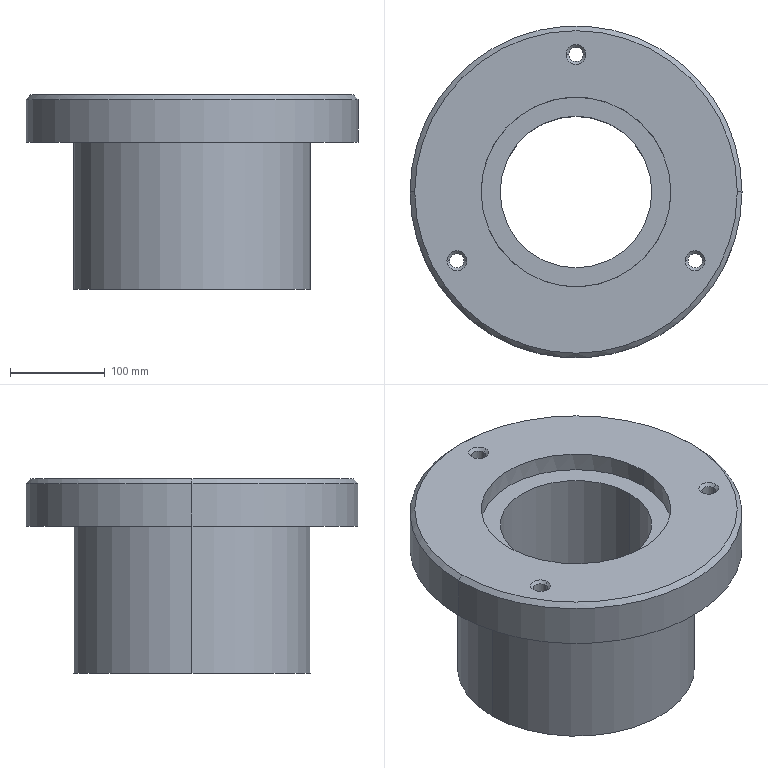Part | SolidWorks | features BaseBody 1 | 1 solid | 26 faces | box 350 x 350 x 205 mm | volume 8030304 mm3 | cylinder 14 | cone 8 | plane 4 | commonest cylinder face diameters 15 x6 160 x2 200 x2 250 x2 350 x2
STEP:
#1=CARTESIAN_POINT('',(165.077,953.249,590.107));
#2=VERTEX_POINT('',#1);
#3=CARTESIAN_POINT('',(165.077,953.249,610.107));
#4=VERTEX_POINT('',#3);
#5=CARTESIAN_POINT('',(165.077,953.249,590.107));
#6=DIRECTION('',(0.,0.,1.));
#7=VECTOR('',#6,1000.);
#8=LINE('',#5,#7);
#9=EDGE_CURVE('',#2,#4,#8,.T.);
#10=ORIENTED_EDGE('',*,*,#9,.F.);
#11=CARTESIAN_POINT('',(365.077,953.249,590.107));
#12=VERTEX_POINT('',#11);
#13=CARTESIAN_POINT('',(265.077,953.249,590.107));
#14=DIRECTION('',(0.,0.,-1.));
#15=DIRECTION('',(-0.9237,-0.383,0.));
#16=AXIS2_PLACEMENT_3D('',#13,#14,#15);
#17=CIRCLE('',#16,100.);
#18=EDGE_CURVE('',#2,#12,#17,.T.);
#19=ORIENTED_EDGE('',*,*,#18,.T.);
#20=CARTESIAN_POINT('',(365.077,953.249,610.107));
#21=VERTEX_POINT('',#20);
#22=CARTESIAN_POINT('',(365.077,953.249,590.107));
#23=DIRECTION('',(0.,0.,1.));
#24=VECTOR('',#23,1000.);
#25=LINE('',#22,#24);
#26=EDGE_CURVE('',#12,#21,#25,.T.);
#27=ORIENTED_EDGE('',*,*,#26,.T.);
#28=CARTESIAN_POINT('',(365.077,953.249,610.107));
#29=CARTESIAN_POINT('',(365.077,959.794,610.107));
#30=CARTESIAN_POINT('',(364.432,966.339,610.107));
#31=CARTESIAN_POINT('',(361.879,979.177,610.107));
#32=CARTESIAN_POINT('',(359.97,985.471,610.107));
#33=CARTESIAN_POINT('',(354.96,997.564,610.107));
#34=CARTESIAN_POINT('',(351.86,1003.364,610.107));
#35=CARTESIAN_POINT('',(344.588,1014.248,610.107));
#36=CARTESIAN_POINT('',(340.416,1019.332,610.107));
#37=CARTESIAN_POINT('',(331.16,1028.588,610.107));
#38=CARTESIAN_POINT('',(326.076,1032.76,610.107));
#39=CARTESIAN_POINT('',(315.192,1040.032,610.107));
#40=CARTESIAN_POINT('',(309.392,1043.132,610.107));
#41=CARTESIAN_POINT('',(297.298,1048.142,610.107));
#42=CARTESIAN_POINT('',(291.005,1050.051,610.107));
#43=CARTESIAN_POINT('',(278.167,1052.604,610.107));
#44=CARTESIAN_POINT('',(271.622,1053.249,610.107));
#45=CARTESIAN_POINT('',(258.532,1053.249,610.107));
#46=CARTESIAN_POINT('',(251.987,1052.604,610.107));
#47=CARTESIAN_POINT('',(239.149,1050.051,610.107));
#48=CARTESIAN_POINT('',(232.855,1048.142,610.107));
#49=CARTESIAN_POINT('',(220.762,1043.132,610.107));
#50=CARTESIAN_POINT('',(214.962,1040.032,610.107));
#51=CARTESIAN_POINT('',(204.078,1032.76,610.107));
#52=CARTESIAN_POINT('',(198.994,1028.588,610.107));
#53=CARTESIAN_POINT('',(189.738,1019.332,610.107));
#54=CARTESIAN_POINT('',(185.566,1014.248,610.107));
#55=CARTESIAN_POINT('',(178.294,1003.364,610.107));
#56=CARTESIAN_POINT('',(175.194,997.564,610.107));
#57=CARTESIAN_POINT('',(170.184,985.471,610.107));
#58=CARTESIAN_POINT('',(168.275,979.177,610.107));
#59=CARTESIAN_POINT('',(165.722,966.339,610.107));
#60=CARTESIAN_POINT('',(165.077,959.794,610.107));
#61=CARTESIAN_POINT('',(165.077,953.249,610.107));
#62=B_SPLINE_CURVE_WITH_KNOTS('',3,(#28,#29,#30,#31,#32,#33,#34,#35,#36,#37,#38,#39,#40,#41,#42,#43,#44,#45,#46,#47,#48,#49,#50,#51,#52,#53,#54,#55,#56,#57,#58,#59,#60,#61),.UNSPECIFIED.,.F.,.F.,(4,2,2,2,2,2,2,2,2,2,2,2,2,2,2,2,4),(0.,0.0625,0.125,0.1875,0.25,0.3125,0.375,0.4375,0.5,0.5625,0.625,0.6875,0.75,0.8125,0.875,0.9375,1.),.UNSPECIFIED.);
#63=EDGE_CURVE('',#21,#4,#62,.T.);
#64=ORIENTED_EDGE('',*,*,#63,.T.);
#65=EDGE_LOOP('',(#10,#19,#27,#64));
#66=FACE_OUTER_BOUND('',#65,.T.);
#67=CARTESIAN_POINT('',(265.077,953.249,590.107));
#68=DIRECTION('',(0.,0.,1.));
#69=DIRECTION('',(1.,0.,0.));
#70=AXIS2_PLACEMENT_3D('',#67,#68,#69);
#71=CYLINDRICAL_SURFACE('',#70,100.);
#72=ADVANCED_FACE('',(#66),#71,.F.);
#73=CARTESIAN_POINT('',(345.077,953.249,590.107));
#74=VERTEX_POINT('',#73);
#75=CARTESIAN_POINT('',(185.077,953.249,590.107));
#76=VERTEX_POINT('',#75);
#77=CARTESIAN_POINT('',(265.077,953.249,590.107));
#78=DIRECTION('',(0.,0.,1.));
#79=DIRECTION('',(-1.,0.,0.));
#80=AXIS2_PLACEMENT_3D('',#77,#78,#79);
#81=CIRCLE('',#80,80.);
#82=EDGE_CURVE('',#74,#76,#81,.T.);
#83=ORIENTED_EDGE('',*,*,#82,.F.);
#84=CARTESIAN_POINT('',(265.077,953.249,590.107));
#85=DIRECTION('',(0.,0.,1.));
#86=DIRECTION('',(-1.,0.,0.));
#87=AXIS2_PLACEMENT_3D('',#84,#85,#86);
#88=CIRCLE('',#87,80.);
#89=EDGE_CURVE('',#76,#74,#88,.T.);
#90=ORIENTED_EDGE('',*,*,#89,.F.);
#91=EDGE_LOOP('',(#83,#90));
#92=FACE_BOUND('',#91,.T.);
#93=CARTESIAN_POINT('',(265.077,953.249,590.107));
#94=DIRECTION('',(0.,0.,-1.));
#95=DIRECTION('',(-0.9237,-0.383,0.));
#96=AXIS2_PLACEMENT_3D('',#93,#94,#95);
#97=CIRCLE('',#96,100.);
#98=EDGE_CURVE('',#12,#2,#97,.T.);
#99=ORIENTED_EDGE('',*,*,#98,.F.);
#100=ORIENTED_EDGE('',*,*,#18,.F.);
#101=EDGE_LOOP('',(#99,#100));
#102=FACE_OUTER_BOUND('',#101,.T.);
#103=CARTESIAN_POINT('',(265.077,953.249,590.107));
#104=DIRECTION('',(0.,0.,-1.));
#105=DIRECTION('',(0.,-1.,0.));
#106=AXIS2_PLACEMENT_3D('',#103,#104,#105);
#107=PLANE('',#106);
#108=ADVANCED_FACE('',(#92,#102),#107,.F.);
#109=CARTESIAN_POINT('',(345.077,953.249,405.107));
#110=VERTEX_POINT('',#109);
#111=CARTESIAN_POINT('',(345.077,953.249,560.107));
#112=DIRECTION('',(0.,0.,-1.));
#113=VECTOR('',#112,1000.);
#114=LINE('',#111,#113);
#115=EDGE_CURVE('',#74,#110,#114,.T.);
#116=ORIENTED_EDGE('',*,*,#115,.F.);
#117=ORIENTED_EDGE('',*,*,#82,.T.);
#118=CARTESIAN_POINT('',(185.077,953.249,405.107));
#119=VERTEX_POINT('',#118);
#120=CARTESIAN_POINT('',(185.077,953.249,560.107));
#121=DIRECTION('',(0.,0.,-1.));
#122=VECTOR('',#121,1000.);
#123=LINE('',#120,#122);
#124=EDGE_CURVE('',#76,#119,#123,.T.);
#125=ORIENTED_EDGE('',*,*,#124,.T.);
#126=CARTESIAN_POINT('',(265.077,953.249,405.107));
#127=DIRECTION('',(0.,0.,1.));
#128=DIRECTION('',(1.,0.,0.));
#129=AXIS2_PLACEMENT_3D('',#126,#127,#128);
#130=CIRCLE('',#129,80.);
#131=EDGE_CURVE('',#110,#119,#130,.T.);
#132=ORIENTED_EDGE('',*,*,#131,.F.);
#133=EDGE_LOOP('',(#116,#117,#125,#132));
#134=FACE_OUTER_BOUND('',#133,.T.);
#135=CARTESIAN_POINT('',(265.077,953.249,560.107));
#136=DIRECTION('',(0.,0.,-1.));
#137=DIRECTION('',(1.,0.,0.));
#138=AXIS2_PLACEMENT_3D('',#135,#136,#137);
#139=CYLINDRICAL_SURFACE('',#138,80.);
#140=ADVANCED_FACE('',(#134),#139,.F.);
#141=ORIENTED_EDGE('',*,*,#124,.F.);
#142=ORIENTED_EDGE('',*,*,#89,.T.);
#143=ORIENTED_EDGE('',*,*,#115,.T.);
#144=CARTESIAN_POINT('',(265.077,953.249,405.107));
#145=DIRECTION('',(0.,0.,1.));
#146=DIRECTION('',(1.,0.,0.));
#147=AXIS2_PLACEMENT_3D('',#144,#145,#146);
#148=CIRCLE('',#147,80.);
#149=EDGE_CURVE('',#119,#110,#148,.T.);
#150=ORIENTED_EDGE('',*,*,#149,.F.);
#151=EDGE_LOOP('',(#141,#142,#143,#150));
#152=FACE_OUTER_BOUND('',#151,.T.);
#153=CARTESIAN_POINT('',(265.077,953.249,560.107));
#154=DIRECTION('',(0.,0.,-1.));
#155=DIRECTION('',(1.,0.,0.));
#156=AXIS2_PLACEMENT_3D('',#153,#154,#155);
#157=CYLINDRICAL_SURFACE('',#156,80.);
#158=ADVANCED_FACE('',(#152),#157,.F.);
#159=ORIENTED_EDGE('',*,*,#149,.T.);
#160=ORIENTED_EDGE('',*,*,#131,.T.);
#161=EDGE_LOOP('',(#159,#160));
#162=FACE_BOUND('',#161,.T.);
#163=CARTESIAN_POINT('',(140.077,953.249,405.107));
#164=VERTEX_POINT('',#163);
#165=CARTESIAN_POINT('',(390.077,953.249,405.107));
#166=VERTEX_POINT('',#165);
#167=CARTESIAN_POINT('',(265.077,953.249,405.107));
#168=DIRECTION('',(0.,0.,1.));
#169=DIRECTION('',(1.,0.,0.));
#170=AXIS2_PLACEMENT_3D('',#167,#168,#169);
#171=CIRCLE('',#170,125.);
#172=EDGE_CURVE('',#164,#166,#171,.T.);
#173=ORIENTED_EDGE('',*,*,#172,.F.);
#174=CARTESIAN_POINT('',(265.077,953.249,405.107));
#175=DIRECTION('',(0.,0.,1.));
#176=DIRECTION('',(1.,0.,0.));
#177=AXIS2_PLACEMENT_3D('',#174,#175,#176);
#178=CIRCLE('',#177,125.);
#179=EDGE_CURVE('',#166,#164,#178,.T.);
#180=ORIENTED_EDGE('',*,*,#179,.F.);
#181=EDGE_LOOP('',(#173,#180));
#182=FACE_OUTER_BOUND('',#181,.T.);
#183=CARTESIAN_POINT('',(265.077,953.249,405.107));
#184=DIRECTION('',(0.,0.,1.));
#185=DIRECTION('',(1.,0.,0.));
#186=AXIS2_PLACEMENT_3D('',#183,#184,#185);
#187=PLANE('',#186);
#188=ADVANCED_FACE('',(#162,#182),#187,.F.);
#189=CARTESIAN_POINT('',(140.077,953.249,560.107));
#190=VERTEX_POINT('',#189);
#191=CARTESIAN_POINT('',(140.077,953.249,610.107));
#192=DIRECTION('',(0.,0.,-1.));
#193=VECTOR('',#192,1000.);
#194=LINE('',#191,#193);
#195=EDGE_CURVE('',#190,#164,#194,.T.);
#196=ORIENTED_EDGE('',*,*,#195,.F.);
#197=CARTESIAN_POINT('',(390.077,953.249,560.107));
#198=VERTEX_POINT('',#197);
#199=CARTESIAN_POINT('',(265.077,953.249,560.107));
#200=DIRECTION('',(0.,0.,1.));
#201=DIRECTION('',(1.,0.,0.));
#202=AXIS2_PLACEMENT_3D('',#199,#200,#201);
#203=CIRCLE('',#202,125.);
#204=EDGE_CURVE('',#198,#190,#203,.T.);
#205=ORIENTED_EDGE('',*,*,#204,.F.);
#206=CARTESIAN_POINT('',(390.077,953.249,610.107));
#207=DIRECTION('',(0.,0.,-1.));
#208=VECTOR('',#207,1000.);
#209=LINE('',#206,#208);
#210=EDGE_CURVE('',#198,#166,#209,.T.);
#211=ORIENTED_EDGE('',*,*,#210,.T.);
#212=ORIENTED_EDGE('',*,*,#179,.T.);
#213=EDGE_LOOP('',(#196,#205,#211,#212));
#214=FACE_OUTER_BOUND('',#213,.T.);
#215=CARTESIAN_POINT('',(265.077,953.249,610.107));
#216=DIRECTION('',(0.,0.,-1.));
#217=DIRECTION('',(1.,0.,0.));
#218=AXIS2_PLACEMENT_3D('',#215,#216,#217);
#219=CYLINDRICAL_SURFACE('',#218,125.);
#220=ADVANCED_FACE('',(#214),#219,.T.);
#221=ORIENTED_EDGE('',*,*,#210,.F.);
#222=CARTESIAN_POINT('',(265.077,953.249,560.107));
#223=DIRECTION('',(0.,0.,1.));
#224=DIRECTION('',(1.,0.,0.));
#225=AXIS2_PLACEMENT_3D('',#222,#223,#224);
#226=CIRCLE('',#225,125.);
#227=EDGE_CURVE('',#190,#198,#226,.T.);
#228=ORIENTED_EDGE('',*,*,#227,.F.);
#229=ORIENTED_EDGE('',*,*,#195,.T.);
#230=ORIENTED_EDGE('',*,*,#172,.T.);
#231=EDGE_LOOP('',(#221,#228,#229,#230));
#232=FACE_OUTER_BOUND('',#231,.T.);
#233=CARTESIAN_POINT('',(265.077,953.249,610.107));
#234=DIRECTION('',(0.,0.,-1.));
#235=DIRECTION('',(1.,0.,0.));
#236=AXIS2_PLACEMENT_3D('',#233,#234,#235);
#237=CYLINDRICAL_SURFACE('',#236,125.);
#238=ADVANCED_FACE('',(#232),#237,.T.);
#239=CARTESIAN_POINT('',(435.077,953.249,610.107));
#240=VERTEX_POINT('',#239);
#241=CARTESIAN_POINT('',(440.077,953.249,605.107));
#242=VERTEX_POINT('',#241);
#243=CARTESIAN_POINT('',(435.077,953.249,610.107));
#244=DIRECTION('',(0.7071,0.,-0.7071));
#245=VECTOR('',#244,1000.);
#246=LINE('',#243,#245);
#247=EDGE_CURVE('',#240,#242,#246,.T.);
#248=ORIENTED_EDGE('',*,*,#247,.F.);
#249=CARTESIAN_POINT('',(95.077,953.249,610.107));
#250=VERTEX_POINT('',#249);
#251=CARTESIAN_POINT('',(265.077,953.249,610.107));
#252=DIRECTION('',(0.,0.,1.));
#253=DIRECTION('',(1.,0.,0.));
#254=AXIS2_PLACEMENT_3D('',#251,#252,#253);
#255=CIRCLE('',#254,170.);
#256=EDGE_CURVE('',#250,#240,#255,.T.);
#257=ORIENTED_EDGE('',*,*,#256,.F.);
#258=CARTESIAN_POINT('',(90.077,953.249,605.107));
#259=VERTEX_POINT('',#258);
#260=CARTESIAN_POINT('',(95.077,953.249,610.107));
#261=DIRECTION('',(-0.7071,0.,-0.7071));
#262=VECTOR('',#261,1000.);
#263=LINE('',#260,#262);
#264=EDGE_CURVE('',#250,#259,#263,.T.);
#265=ORIENTED_EDGE('',*,*,#264,.T.);
#266=CARTESIAN_POINT('',(265.077,953.249,605.107));
#267=DIRECTION('',(0.,0.,-1.));
#268=DIRECTION('',(1.,0.,0.));
#269=AXIS2_PLACEMENT_3D('',#266,#267,#268);
#270=CIRCLE('',#269,175.);
#271=EDGE_CURVE('',#242,#259,#270,.T.);
#272=ORIENTED_EDGE('',*,*,#271,.F.);
#273=EDGE_LOOP('',(#248,#257,#265,#272));
#274=FACE_OUTER_BOUND('',#273,.T.);
#275=CARTESIAN_POINT('',(265.077,953.249,610.107));
#276=DIRECTION('',(0.,0.,-1.));
#277=DIRECTION('',(1.,0.,0.));
#278=AXIS2_PLACEMENT_3D('',#275,#276,#277);
#279=CONICAL_SURFACE('',#278,170.,0.7854);
#280=ADVANCED_FACE('',(#274),#279,.T.);
#281=CARTESIAN_POINT('',(257.577,1098.249,607.107));
#282=VERTEX_POINT('',#281);
#283=CARTESIAN_POINT('',(254.577,1098.249,610.107));
#284=VERTEX_POINT('',#283);
#285=CARTESIAN_POINT('',(257.577,1098.249,607.107));
#286=DIRECTION('',(-0.7071,0.,0.7071));
#287=VECTOR('',#286,1000.);
#288=LINE('',#285,#287);
#289=EDGE_CURVE('',#282,#284,#288,.T.);
#290=ORIENTED_EDGE('',*,*,#289,.F.);
#291=CARTESIAN_POINT('',(272.577,1098.249,607.107));
#292=VERTEX_POINT('',#291);
#293=CARTESIAN_POINT('',(265.077,1098.249,607.107));
#294=DIRECTION('',(0.,0.,1.));
#295=DIRECTION('',(1.,0.,0.));
#296=AXIS2_PLACEMENT_3D('',#293,#294,#295);
#297=CIRCLE('',#296,7.5);
#298=EDGE_CURVE('',#292,#282,#297,.T.);
#299=ORIENTED_EDGE('',*,*,#298,.F.);
#300=CARTESIAN_POINT('',(275.577,1098.249,610.107));
#301=VERTEX_POINT('',#300);
#302=CARTESIAN_POINT('',(272.577,1098.249,607.107));
#303=DIRECTION('',(0.7071,0.,0.7071));
#304=VECTOR('',#303,1000.);
#305=LINE('',#302,#304);
#306=EDGE_CURVE('',#292,#301,#305,.T.);
#307=ORIENTED_EDGE('',*,*,#306,.T.);
#308=CARTESIAN_POINT('',(265.077,1098.249,610.107));
#309=DIRECTION('',(0.,0.,-1.));
#310=DIRECTION('',(1.,0.,0.));
#311=AXIS2_PLACEMENT_3D('',#308,#309,#310);
#312=CIRCLE('',#311,10.5);
#313=EDGE_CURVE('',#284,#301,#312,.T.);
#314=ORIENTED_EDGE('',*,*,#313,.F.);
#315=EDGE_LOOP('',(#290,#299,#307,#314));
#316=FACE_OUTER_BOUND('',#315,.T.);
#317=CARTESIAN_POINT('',(265.077,1098.249,607.107));
#318=DIRECTION('',(0.,0.,1.));
#319=DIRECTION('',(-1.,0.,0.));
#320=AXIS2_PLACEMENT_3D('',#317,#318,#319);
#321=CONICAL_SURFACE('',#320,7.5,0.7854);
#322=ADVANCED_FACE('',(#316),#321,.F.);
#323=CARTESIAN_POINT('',(132.003,880.749,607.107));
#324=VERTEX_POINT('',#323);
#325=CARTESIAN_POINT('',(129.003,880.749,610.107));
#326=VERTEX_POINT('',#325);
#327=CARTESIAN_POINT('',(132.003,880.749,607.107));
#328=DIRECTION('',(-0.7071,0.,0.7071));
#329=VECTOR('',#328,1000.);
#330=LINE('',#327,#329);
#331=EDGE_CURVE('',#324,#326,#330,.T.);
#332=ORIENTED_EDGE('',*,*,#331,.F.);
#333=CARTESIAN_POINT('',(147.003,880.749,607.107));
#334=VERTEX_POINT('',#333);
#335=CARTESIAN_POINT('',(139.503,880.749,607.107));
#336=DIRECTION('',(0.,0.,1.));
#337=DIRECTION('',(1.,0.,0.));
#338=AXIS2_PLACEMENT_3D('',#335,#336,#337);
#339=CIRCLE('',#338,7.5);
#340=EDGE_CURVE('',#334,#324,#339,.T.);
#341=ORIENTED_EDGE('',*,*,#340,.F.);
#342=CARTESIAN_POINT('',(150.003,880.749,610.107));
#343=VERTEX_POINT('',#342);
#344=CARTESIAN_POINT('',(147.003,880.749,607.107));
#345=DIRECTION('',(0.7071,0.,0.7071));
#346=VECTOR('',#345,1000.);
#347=LINE('',#344,#346);
#348=EDGE_CURVE('',#334,#343,#347,.T.);
#349=ORIENTED_EDGE('',*,*,#348,.T.);
#350=CARTESIAN_POINT('',(139.503,880.749,610.107));
#351=DIRECTION('',(0.,0.,-1.));
#352=DIRECTION('',(1.,0.,0.));
#353=AXIS2_PLACEMENT_3D('',#350,#351,#352);
#354=CIRCLE('',#353,10.5);
#355=EDGE_CURVE('',#326,#343,#354,.T.);
#356=ORIENTED_EDGE('',*,*,#355,.F.);
#357=EDGE_LOOP('',(#332,#341,#349,#356));
#358=FACE_OUTER_BOUND('',#357,.T.);
#359=CARTESIAN_POINT('',(139.503,880.749,607.107));
#360=DIRECTION('',(0.,0.,1.));
#361=DIRECTION('',(-1.,0.,0.));
#362=AXIS2_PLACEMENT_3D('',#359,#360,#361);
#363=CONICAL_SURFACE('',#362,7.5,0.7854);
#364=ADVANCED_FACE('',(#358),#363,.F.);
#365=CARTESIAN_POINT('',(383.151,880.749,607.107));
#366=VERTEX_POINT('',#365);
#367=CARTESIAN_POINT('',(380.151,880.749,610.107));
#368=VERTEX_POINT('',#367);
#369=CARTESIAN_POINT('',(383.151,880.749,607.107));
#370=DIRECTION('',(-0.7071,0.,0.7071));
#371=VECTOR('',#370,1000.);
#372=LINE('',#369,#371);
#373=EDGE_CURVE('',#366,#368,#372,.T.);
#374=ORIENTED_EDGE('',*,*,#373,.F.);
#375=CARTESIAN_POINT('',(398.151,880.749,607.107));
#376=VERTEX_POINT('',#375);
#377=CARTESIAN_POINT('',(390.651,880.749,607.107));
#378=DIRECTION('',(0.,0.,1.));
#379=DIRECTION('',(1.,0.,0.));
#380=AXIS2_PLACEMENT_3D('',#377,#378,#379);
#381=CIRCLE('',#380,7.5);
#382=EDGE_CURVE('',#376,#366,#381,.T.);
#383=ORIENTED_EDGE('',*,*,#382,.F.);
#384=CARTESIAN_POINT('',(401.151,880.749,610.107));
#385=VERTEX_POINT('',#384);
#386=CARTESIAN_POINT('',(398.151,880.749,607.107));
#387=DIRECTION('',(0.7071,0.,0.7071));
#388=VECTOR('',#387,1000.);
#389=LINE('',#386,#388);
#390=EDGE_CURVE('',#376,#385,#389,.T.);
#391=ORIENTED_EDGE('',*,*,#390,.T.);
#392=CARTESIAN_POINT('',(390.651,880.749,610.107));
#393=DIRECTION('',(0.,0.,-1.));
#394=DIRECTION('',(1.,0.,0.));
#395=AXIS2_PLACEMENT_3D('',#392,#393,#394);
#396=CIRCLE('',#395,10.5);
#397=EDGE_CURVE('',#368,#385,#396,.T.);
#398=ORIENTED_EDGE('',*,*,#397,.F.);
#399=EDGE_LOOP('',(#374,#383,#391,#398));
#400=FACE_OUTER_BOUND('',#399,.T.);
#401=CARTESIAN_POINT('',(390.651,880.749,607.107));
#402=DIRECTION('',(0.,0.,1.));
#403=DIRECTION('',(-1.,0.,0.));
#404=AXIS2_PLACEMENT_3D('',#401,#402,#403);
#405=CONICAL_SURFACE('',#404,7.5,0.7854);
#406=ADVANCED_FACE('',(#400),#405,.F.);
#407=CARTESIAN_POINT('',(132.003,880.749,560.107));
#408=VERTEX_POINT('',#407);
#409=CARTESIAN_POINT('',(132.003,880.749,538.893));
#410=DIRECTION('',(0.,0.,1.));
#411=VECTOR('',#410,1000.);
#412=LINE('',#409,#411);
#413=EDGE_CURVE('',#408,#324,#412,.T.);
#414=ORIENTED_EDGE('',*,*,#413,.F.);
#415=CARTESIAN_POINT('',(147.003,880.749,560.107));
#416=VERTEX_POINT('',#415);
#417=CARTESIAN_POINT('',(139.503,880.749,560.107));
#418=DIRECTION('',(0.,0.,-1.));
#419=DIRECTION('',(1.,0.,0.));
#420=AXIS2_PLACEMENT_3D('',#417,#418,#419);
#421=CIRCLE('',#420,7.5);
#422=EDGE_CURVE('',#408,#416,#421,.T.);
#423=ORIENTED_EDGE('',*,*,#422,.T.);
#424=CARTESIAN_POINT('',(147.003,880.749,538.893));
#425=DIRECTION('',(0.,0.,1.));
#426=VECTOR('',#425,1000.);
#427=LINE('',#424,#426);
#428=EDGE_CURVE('',#416,#334,#427,.T.);
#429=ORIENTED_EDGE('',*,*,#428,.T.);
#430=ORIENTED_EDGE('',*,*,#340,.T.);
#431=EDGE_LOOP('',(#414,#423,#429,#430));
#432=FACE_OUTER_BOUND('',#431,.T.);
#433=CARTESIAN_POINT('',(139.503,880.749,538.893));
#434=DIRECTION('',(0.,0.,1.));
#435=DIRECTION('',(-1.,0.,0.));
#436=AXIS2_PLACEMENT_3D('',#433,#434,#435);
#437=CYLINDRICAL_SURFACE('',#436,7.5);
#438=ADVANCED_FACE('',(#432),#437,.F.);
#439=CARTESIAN_POINT('',(383.151,880.749,560.107));
#440=VERTEX_POINT('',#439);
#441=CARTESIAN_POINT('',(383.151,880.749,538.893));
#442=DIRECTION('',(0.,0.,1.));
#443=VECTOR('',#442,1000.);
#444=LINE('',#441,#443);
#445=EDGE_CURVE('',#440,#366,#444,.T.);
#446=ORIENTED_EDGE('',*,*,#445,.F.);
#447=CARTESIAN_POINT('',(398.151,880.749,560.107));
#448=VERTEX_POINT('',#447);
#449=CARTESIAN_POINT('',(390.651,880.749,560.107));
#450=DIRECTION('',(0.,0.,-1.));
#451=DIRECTION('',(1.,0.,0.));
#452=AXIS2_PLACEMENT_3D('',#449,#450,#451);
#453=CIRCLE('',#452,7.5);
#454=EDGE_CURVE('',#440,#448,#453,.T.);
#455=ORIENTED_EDGE('',*,*,#454,.T.);
#456=CARTESIAN_POINT('',(398.151,880.749,538.893));
#457=DIRECTION('',(0.,0.,1.));
#458=VECTOR('',#457,1000.);
#459=LINE('',#456,#458);
#460=EDGE_CURVE('',#448,#376,#459,.T.);
#461=ORIENTED_EDGE('',*,*,#460,.T.);
#462=ORIENTED_EDGE('',*,*,#382,.T.);
#463=EDGE_LOOP('',(#446,#455,#461,#462));
#464=FACE_OUTER_BOUND('',#463,.T.);
#465=CARTESIAN_POINT('',(390.651,880.749,538.893));
#466=DIRECTION('',(0.,0.,1.));
#467=DIRECTION('',(-1.,0.,0.));
#468=AXIS2_PLACEMENT_3D('',#465,#466,#467);
#469=CYLINDRICAL_SURFACE('',#468,7.5);
#470=ADVANCED_FACE('',(#464),#469,.F.);
#471=CARTESIAN_POINT('',(257.577,1098.249,560.107));
#472=VERTEX_POINT('',#471);
#473=CARTESIAN_POINT('',(257.577,1098.249,538.893));
#474=DIRECTION('',(0.,0.,1.));
#475=VECTOR('',#474,1000.);
#476=LINE('',#473,#475);
#477=EDGE_CURVE('',#472,#282,#476,.T.);
#478=ORIENTED_EDGE('',*,*,#477,.F.);
#479=CARTESIAN_POINT('',(272.577,1098.249,560.107));
#480=VERTEX_POINT('',#479);
#481=CARTESIAN_POINT('',(265.077,1098.249,560.107));
#482=DIRECTION('',(0.,0.,-1.));
#483=DIRECTION('',(1.,0.,0.));
#484=AXIS2_PLACEMENT_3D('',#481,#482,#483);
#485=CIRCLE('',#484,7.5);
#486=EDGE_CURVE('',#472,#480,#485,.T.);
#487=ORIENTED_EDGE('',*,*,#486,.T.);
#488=CARTESIAN_POINT('',(272.577,1098.249,538.893));
#489=DIRECTION('',(0.,0.,1.));
#490=VECTOR('',#489,1000.);
#491=LINE('',#488,#490);
#492=EDGE_CURVE('',#480,#292,#491,.T.);
#493=ORIENTED_EDGE('',*,*,#492,.T.);
#494=ORIENTED_EDGE('',*,*,#298,.T.);
#495=EDGE_LOOP('',(#478,#487,#493,#494));
#496=FACE_OUTER_BOUND('',#495,.T.);
#497=CARTESIAN_POINT('',(265.077,1098.249,538.893));
#498=DIRECTION('',(0.,0.,1.));
#499=DIRECTION('',(-1.,0.,0.));
#500=AXIS2_PLACEMENT_3D('',#497,#498,#499);
#501=CYLINDRICAL_SURFACE('',#500,7.5);
#502=ADVANCED_FACE('',(#496),#501,.F.);
#503=ORIENTED_EDGE('',*,*,#63,.F.);
#504=CARTESIAN_POINT('',(165.077,953.249,610.107));
#505=CARTESIAN_POINT('',(165.077,946.704,610.107));
#506=CARTESIAN_POINT('',(165.722,940.159,610.107));
#507=CARTESIAN_POINT('',(168.275,927.321,610.107));
#508=CARTESIAN_POINT('',(170.184,921.027,610.107));
#509=CARTESIAN_POINT('',(175.194,908.934,610.107));
#510=CARTESIAN_POINT('',(178.294,903.134,610.107));
#511=CARTESIAN_POINT('',(185.566,892.25,610.107));
#512=CARTESIAN_POINT('',(189.738,887.166,610.107));
#513=CARTESIAN_POINT('',(198.994,877.91,610.107));
#514=CARTESIAN_POINT('',(204.078,873.738,610.107));
#515=CARTESIAN_POINT('',(214.962,866.466,610.107));
#516=CARTESIAN_POINT('',(220.762,863.366,610.107));
#517=CARTESIAN_POINT('',(232.855,858.356,610.107));
#518=CARTESIAN_POINT('',(239.149,856.447,610.107));
#519=CARTESIAN_POINT('',(251.987,853.894,610.107));
#520=CARTESIAN_POINT('',(258.532,853.249,610.107));
#521=CARTESIAN_POINT('',(271.622,853.249,610.107));
#522=CARTESIAN_POINT('',(278.167,853.894,610.107));
#523=CARTESIAN_POINT('',(291.005,856.447,610.107));
#524=CARTESIAN_POINT('',(297.298,858.356,610.107));
#525=CARTESIAN_POINT('',(309.392,863.366,610.107));
#526=CARTESIAN_POINT('',(315.192,866.466,610.107));
#527=CARTESIAN_POINT('',(326.076,873.738,610.107));
#528=CARTESIAN_POINT('',(331.16,877.91,610.107));
#529=CARTESIAN_POINT('',(340.416,887.166,610.107));
#530=CARTESIAN_POINT('',(344.588,892.25,610.107));
#531=CARTESIAN_POINT('',(351.86,903.134,610.107));
#532=CARTESIAN_POINT('',(354.96,908.934,610.107));
#533=CARTESIAN_POINT('',(359.97,921.027,610.107));
#534=CARTESIAN_POINT('',(361.879,927.321,610.107));
#535=CARTESIAN_POINT('',(364.432,940.159,610.107));
#536=CARTESIAN_POINT('',(365.077,946.704,610.107));
#537=CARTESIAN_POINT('',(365.077,953.249,610.107));
#538=B_SPLINE_CURVE_WITH_KNOTS('',3,(#504,#505,#506,#507,#508,#509,#510,#511,#512,#513,#514,#515,#516,#517,#518,#519,#520,#521,#522,#523,#524,#525,#526,#527,#528,#529,#530,#531,#532,#533,#534,#535,#536,#537),.UNSPECIFIED.,.F.,.F.,(4,2,2,2,2,2,2,2,2,2,2,2,2,2,2,2,4),(0.,0.0625,0.125,0.1875,0.25,0.3125,0.375,0.4375,0.5,0.5625,0.625,0.6875,0.75,0.8125,0.875,0.9375,1.),.UNSPECIFIED.);
#539=EDGE_CURVE('',#4,#21,#538,.T.);
#540=ORIENTED_EDGE('',*,*,#539,.F.);
#541=EDGE_LOOP('',(#503,#540));
#542=FACE_BOUND('',#541,.T.);
#543=CARTESIAN_POINT('',(265.077,1098.249,610.107));
#544=DIRECTION('',(0.,0.,-1.));
#545=DIRECTION('',(1.,0.,0.));
#546=AXIS2_PLACEMENT_3D('',#543,#544,#545);
#547=CIRCLE('',#546,10.5);
#548=EDGE_CURVE('',#301,#284,#547,.T.);
#549=ORIENTED_EDGE('',*,*,#548,.T.);
#550=ORIENTED_EDGE('',*,*,#313,.T.);
#551=EDGE_LOOP('',(#549,#550));
#552=FACE_BOUND('',#551,.T.);
#553=CARTESIAN_POINT('',(139.503,880.749,610.107));
#554=DIRECTION('',(0.,0.,-1.));
#555=DIRECTION('',(1.,0.,0.));
#556=AXIS2_PLACEMENT_3D('',#553,#554,#555);
#557=CIRCLE('',#556,10.5);
#558=EDGE_CURVE('',#343,#326,#557,.T.);
#559=ORIENTED_EDGE('',*,*,#558,.T.);
#560=ORIENTED_EDGE('',*,*,#355,.T.);
#561=EDGE_LOOP('',(#559,#560));
#562=FACE_BOUND('',#561,.T.);
#563=CARTESIAN_POINT('',(390.651,880.749,610.107));
#564=DIRECTION('',(0.,0.,-1.));
#565=DIRECTION('',(1.,0.,0.));
#566=AXIS2_PLACEMENT_3D('',#563,#564,#565);
#567=CIRCLE('',#566,10.5);
#568=EDGE_CURVE('',#385,#368,#567,.T.);
#569=ORIENTED_EDGE('',*,*,#568,.T.);
#570=ORIENTED_EDGE('',*,*,#397,.T.);
#571=EDGE_LOOP('',(#569,#570));
#572=FACE_BOUND('',#571,.T.);
#573=ORIENTED_EDGE('',*,*,#256,.T.);
#574=CARTESIAN_POINT('',(265.077,953.249,610.107));
#575=DIRECTION('',(0.,0.,1.));
#576=DIRECTION('',(1.,0.,0.));
#577=AXIS2_PLACEMENT_3D('',#574,#575,#576);
#578=CIRCLE('',#577,170.);
#579=EDGE_CURVE('',#240,#250,#578,.T.);
#580=ORIENTED_EDGE('',*,*,#579,.T.);
#581=EDGE_LOOP('',(#573,#580));
#582=FACE_OUTER_BOUND('',#581,.T.);
#583=CARTESIAN_POINT('',(265.077,953.249,610.107));
#584=DIRECTION('',(0.,0.,1.));
#585=DIRECTION('',(1.,0.,0.));
#586=AXIS2_PLACEMENT_3D('',#583,#584,#585);
#587=PLANE('',#586);
#588=ADVANCED_FACE('',(#542,#552,#562,#572,#582),#587,.T.);
#589=CARTESIAN_POINT('',(440.077,953.249,560.107));
#590=VERTEX_POINT('',#589);
#591=CARTESIAN_POINT('',(440.077,953.249,610.107));
#592=DIRECTION('',(0.,0.,-1.));
#593=VECTOR('',#592,1000.);
#594=LINE('',#591,#593);
#595=EDGE_CURVE('',#242,#590,#594,.T.);
#596=ORIENTED_EDGE('',*,*,#595,.F.);
#597=ORIENTED_EDGE('',*,*,#271,.T.);
#598=CARTESIAN_POINT('',(90.077,953.249,560.107));
#599=VERTEX_POINT('',#598);
#600=CARTESIAN_POINT('',(90.077,953.249,610.107));
#601=DIRECTION('',(0.,0.,-1.));
#602=VECTOR('',#601,1000.);
#603=LINE('',#600,#602);
#604=EDGE_CURVE('',#259,#599,#603,.T.);
#605=ORIENTED_EDGE('',*,*,#604,.T.);
#606=CARTESIAN_POINT('',(265.077,953.249,560.107));
#607=DIRECTION('',(0.,0.,1.));
#608=DIRECTION('',(1.,0.,0.));
#609=AXIS2_PLACEMENT_3D('',#606,#607,#608);
#610=CIRCLE('',#609,175.);
#611=EDGE_CURVE('',#599,#590,#610,.T.);
#612=ORIENTED_EDGE('',*,*,#611,.T.);
#613=EDGE_LOOP('',(#596,#597,#605,#612));
#614=FACE_OUTER_BOUND('',#613,.T.);
#615=CARTESIAN_POINT('',(265.077,953.249,610.107));
#616=DIRECTION('',(0.,0.,-1.));
#617=DIRECTION('',(1.,0.,0.));
#618=AXIS2_PLACEMENT_3D('',#615,#616,#617);
#619=CYLINDRICAL_SURFACE('',#618,175.);
#620=ADVANCED_FACE('',(#614),#619,.T.);
#621=ORIENTED_EDGE('',*,*,#204,.T.);
#622=ORIENTED_EDGE('',*,*,#227,.T.);
#623=EDGE_LOOP('',(#621,#622));
#624=FACE_BOUND('',#623,.T.);
#625=CARTESIAN_POINT('',(265.077,1098.249,560.107));
#626=DIRECTION('',(0.,0.,-1.));
#627=DIRECTION('',(1.,0.,0.));
#628=AXIS2_PLACEMENT_3D('',#625,#626,#627);
#629=CIRCLE('',#628,7.5);
#630=EDGE_CURVE('',#480,#472,#629,.T.);
#631=ORIENTED_EDGE('',*,*,#630,.F.);
#632=ORIENTED_EDGE('',*,*,#486,.F.);
#633=EDGE_LOOP('',(#631,#632));
#634=FACE_BOUND('',#633,.T.);
#635=CARTESIAN_POINT('',(390.651,880.749,560.107));
#636=DIRECTION('',(0.,0.,-1.));
#637=DIRECTION('',(1.,0.,0.));
#638=AXIS2_PLACEMENT_3D('',#635,#636,#637);
#639=CIRCLE('',#638,7.5);
#640=EDGE_CURVE('',#448,#440,#639,.T.);
#641=ORIENTED_EDGE('',*,*,#640,.F.);
#642=ORIENTED_EDGE('',*,*,#454,.F.);
#643=EDGE_LOOP('',(#641,#642));
#644=FACE_BOUND('',#643,.T.);
#645=CARTESIAN_POINT('',(139.503,880.749,560.107));
#646=DIRECTION('',(0.,0.,-1.));
#647=DIRECTION('',(1.,0.,0.));
#648=AXIS2_PLACEMENT_3D('',#645,#646,#647);
#649=CIRCLE('',#648,7.5);
#650=EDGE_CURVE('',#416,#408,#649,.T.);
#651=ORIENTED_EDGE('',*,*,#650,.F.);
#652=ORIENTED_EDGE('',*,*,#422,.F.);
#653=EDGE_LOOP('',(#651,#652));
#654=FACE_BOUND('',#653,.T.);
#655=ORIENTED_EDGE('',*,*,#611,.F.);
#656=CARTESIAN_POINT('',(265.077,953.249,560.107));
#657=DIRECTION('',(0.,0.,1.));
#658=DIRECTION('',(1.,0.,0.));
#659=AXIS2_PLACEMENT_3D('',#656,#657,#658);
#660=CIRCLE('',#659,175.);
#661=EDGE_CURVE('',#590,#599,#660,.T.);
#662=ORIENTED_EDGE('',*,*,#661,.F.);
#663=EDGE_LOOP('',(#655,#662));
#664=FACE_OUTER_BOUND('',#663,.T.);
#665=CARTESIAN_POINT('',(265.077,953.249,560.107));
#666=DIRECTION('',(0.,0.,1.));
#667=DIRECTION('',(1.,0.,0.));
#668=AXIS2_PLACEMENT_3D('',#665,#666,#667);
#669=PLANE('',#668);
#670=ADVANCED_FACE('',(#624,#634,#644,#654,#664),#669,.F.);
#671=CARTESIAN_POINT('',(265.077,953.249,605.107));
#672=DIRECTION('',(0.,0.,-1.));
#673=DIRECTION('',(1.,0.,0.));
#674=AXIS2_PLACEMENT_3D('',#671,#672,#673);
#675=CIRCLE('',#674,175.);
#676=EDGE_CURVE('',#259,#242,#675,.T.);
#677=ORIENTED_EDGE('',*,*,#676,.T.);
#678=ORIENTED_EDGE('',*,*,#595,.T.);
#679=ORIENTED_EDGE('',*,*,#661,.T.);
#680=ORIENTED_EDGE('',*,*,#604,.F.);
#681=EDGE_LOOP('',(#677,#678,#679,#680));
#682=FACE_OUTER_BOUND('',#681,.T.);
#683=CARTESIAN_POINT('',(265.077,953.249,610.107));
#684=DIRECTION('',(0.,0.,-1.));
#685=DIRECTION('',(1.,0.,0.));
#686=AXIS2_PLACEMENT_3D('',#683,#684,#685);
#687=CYLINDRICAL_SURFACE('',#686,175.);
#688=ADVANCED_FACE('',(#682),#687,.T.);
#689=ORIENTED_EDGE('',*,*,#630,.T.);
#690=ORIENTED_EDGE('',*,*,#477,.T.);
#691=CARTESIAN_POINT('',(265.077,1098.249,607.107));
#692=DIRECTION('',(0.,0.,1.));
#693=DIRECTION('',(1.,0.,0.));
#694=AXIS2_PLACEMENT_3D('',#691,#692,#693);
#695=CIRCLE('',#694,7.5);
#696=EDGE_CURVE('',#282,#292,#695,.T.);
#697=ORIENTED_EDGE('',*,*,#696,.T.);
#698=ORIENTED_EDGE('',*,*,#492,.F.);
#699=EDGE_LOOP('',(#689,#690,#697,#698));
#700=FACE_OUTER_BOUND('',#699,.T.);
#701=CARTESIAN_POINT('',(265.077,1098.249,538.893));
#702=DIRECTION('',(0.,0.,1.));
#703=DIRECTION('',(-1.,0.,0.));
#704=AXIS2_PLACEMENT_3D('',#701,#702,#703);
#705=CYLINDRICAL_SURFACE('',#704,7.5);
#706=ADVANCED_FACE('',(#700),#705,.F.);
#707=ORIENTED_EDGE('',*,*,#640,.T.);
#708=ORIENTED_EDGE('',*,*,#445,.T.);
#709=CARTESIAN_POINT('',(390.651,880.749,607.107));
#710=DIRECTION('',(0.,0.,1.));
#711=DIRECTION('',(1.,0.,0.));
#712=AXIS2_PLACEMENT_3D('',#709,#710,#711);
#713=CIRCLE('',#712,7.5);
#714=EDGE_CURVE('',#366,#376,#713,.T.);
#715=ORIENTED_EDGE('',*,*,#714,.T.);
#716=ORIENTED_EDGE('',*,*,#460,.F.);
#717=EDGE_LOOP('',(#707,#708,#715,#716));
#718=FACE_OUTER_BOUND('',#717,.T.);
#719=CARTESIAN_POINT('',(390.651,880.749,538.893));
#720=DIRECTION('',(0.,0.,1.));
#721=DIRECTION('',(-1.,0.,0.));
#722=AXIS2_PLACEMENT_3D('',#719,#720,#721);
#723=CYLINDRICAL_SURFACE('',#722,7.5);
#724=ADVANCED_FACE('',(#718),#723,.F.);
#725=ORIENTED_EDGE('',*,*,#650,.T.);
#726=ORIENTED_EDGE('',*,*,#413,.T.);
#727=CARTESIAN_POINT('',(139.503,880.749,607.107));
#728=DIRECTION('',(0.,0.,1.));
#729=DIRECTION('',(1.,0.,0.));
#730=AXIS2_PLACEMENT_3D('',#727,#728,#729);
#731=CIRCLE('',#730,7.5);
#732=EDGE_CURVE('',#324,#334,#731,.T.);
#733=ORIENTED_EDGE('',*,*,#732,.T.);
#734=ORIENTED_EDGE('',*,*,#428,.F.);
#735=EDGE_LOOP('',(#725,#726,#733,#734));
#736=FACE_OUTER_BOUND('',#735,.T.);
#737=CARTESIAN_POINT('',(139.503,880.749,538.893));
#738=DIRECTION('',(0.,0.,1.));
#739=DIRECTION('',(-1.,0.,0.));
#740=AXIS2_PLACEMENT_3D('',#737,#738,#739);
#741=CYLINDRICAL_SURFACE('',#740,7.5);
#742=ADVANCED_FACE('',(#736),#741,.F.);
#743=ORIENTED_EDGE('',*,*,#714,.F.);
#744=ORIENTED_EDGE('',*,*,#373,.T.);
#745=ORIENTED_EDGE('',*,*,#568,.F.);
#746=ORIENTED_EDGE('',*,*,#390,.F.);
#747=EDGE_LOOP('',(#743,#744,#745,#746));
#748=FACE_OUTER_BOUND('',#747,.T.);
#749=CARTESIAN_POINT('',(390.651,880.749,607.107));
#750=DIRECTION('',(0.,0.,1.));
#751=DIRECTION('',(-1.,0.,0.));
#752=AXIS2_PLACEMENT_3D('',#749,#750,#751);
#753=CONICAL_SURFACE('',#752,7.5,0.7854);
#754=ADVANCED_FACE('',(#748),#753,.F.);
#755=ORIENTED_EDGE('',*,*,#732,.F.);
#756=ORIENTED_EDGE('',*,*,#331,.T.);
#757=ORIENTED_EDGE('',*,*,#558,.F.);
#758=ORIENTED_EDGE('',*,*,#348,.F.);
#759=EDGE_LOOP('',(#755,#756,#757,#758));
#760=FACE_OUTER_BOUND('',#759,.T.);
#761=CARTESIAN_POINT('',(139.503,880.749,607.107));
#762=DIRECTION('',(0.,0.,1.));
#763=DIRECTION('',(-1.,0.,0.));
#764=AXIS2_PLACEMENT_3D('',#761,#762,#763);
#765=CONICAL_SURFACE('',#764,7.5,0.7854);
#766=ADVANCED_FACE('',(#760),#765,.F.);
#767=ORIENTED_EDGE('',*,*,#696,.F.);
#768=ORIENTED_EDGE('',*,*,#289,.T.);
#769=ORIENTED_EDGE('',*,*,#548,.F.);
#770=ORIENTED_EDGE('',*,*,#306,.F.);
#771=EDGE_LOOP('',(#767,#768,#769,#770));
#772=FACE_OUTER_BOUND('',#771,.T.);
#773=CARTESIAN_POINT('',(265.077,1098.249,607.107));
#774=DIRECTION('',(0.,0.,1.));
#775=DIRECTION('',(-1.,0.,0.));
#776=AXIS2_PLACEMENT_3D('',#773,#774,#775);
#777=CONICAL_SURFACE('',#776,7.5,0.7854);
#778=ADVANCED_FACE('',(#772),#777,.F.);
#779=ORIENTED_EDGE('',*,*,#579,.F.);
#780=ORIENTED_EDGE('',*,*,#247,.T.);
#781=ORIENTED_EDGE('',*,*,#676,.F.);
#782=ORIENTED_EDGE('',*,*,#264,.F.);
#783=EDGE_LOOP('',(#779,#780,#781,#782));
#784=FACE_OUTER_BOUND('',#783,.T.);
#785=CARTESIAN_POINT('',(265.077,953.249,610.107));
#786=DIRECTION('',(0.,0.,-1.));
#787=DIRECTION('',(1.,0.,0.));
#788=AXIS2_PLACEMENT_3D('',#785,#786,#787);
#789=CONICAL_SURFACE('',#788,170.,0.7854);
#790=ADVANCED_FACE('',(#784),#789,.T.);
#791=ORIENTED_EDGE('',*,*,#98,.T.);
#792=ORIENTED_EDGE('',*,*,#9,.T.);
#793=ORIENTED_EDGE('',*,*,#539,.T.);
#794=ORIENTED_EDGE('',*,*,#26,.F.);
#795=EDGE_LOOP('',(#791,#792,#793,#794));
#796=FACE_OUTER_BOUND('',#795,.T.);
#797=CARTESIAN_POINT('',(265.077,953.249,590.107));
#798=DIRECTION('',(0.,0.,1.));
#799=DIRECTION('',(1.,0.,0.));
#800=AXIS2_PLACEMENT_3D('',#797,#798,#799);
#801=CYLINDRICAL_SURFACE('',#800,100.);
#802=ADVANCED_FACE('',(#796),#801,.F.);
#803=CLOSED_SHELL('',(#72,#108,#140,#158,#188,#220,#238,#280,#322,#364,#406,#438,#470,#502,#588,#620,#670,#688,#706,#724,#742,#754,#766,#778,#790,#802));
#804=MANIFOLD_SOLID_BREP('',#803);
#805=CARTESIAN_POINT('',(0.,0.,0.));
#806=DIRECTION('',(0.,0.,1.));
#807=DIRECTION('',(1.,0.,0.));
#808=AXIS2_PLACEMENT_3D('',#805,#806,#807);
#809=(LENGTH_UNIT()NAMED_UNIT(*)SI_UNIT(.MILLI.,.METRE.));
#810=UNCERTAINTY_MEASURE_WITH_UNIT(LENGTH_MEASURE(0.00001),#809,'','');
#811=(NAMED_UNIT(*)PLANE_ANGLE_UNIT()SI_UNIT($,.RADIAN.));
#812=(NAMED_UNIT(*)SI_UNIT($,.STERADIAN.)SOLID_ANGLE_UNIT());
#813=(GEOMETRIC_REPRESENTATION_CONTEXT(3)GLOBAL_UNCERTAINTY_ASSIGNED_CONTEXT((#810))GLOBAL_UNIT_ASSIGNED_CONTEXT((#809,#811,#812))REPRESENTATION_CONTEXT('',''));
#814=ADVANCED_BREP_SHAPE_REPRESENTATION('',(#804,#808),#813);